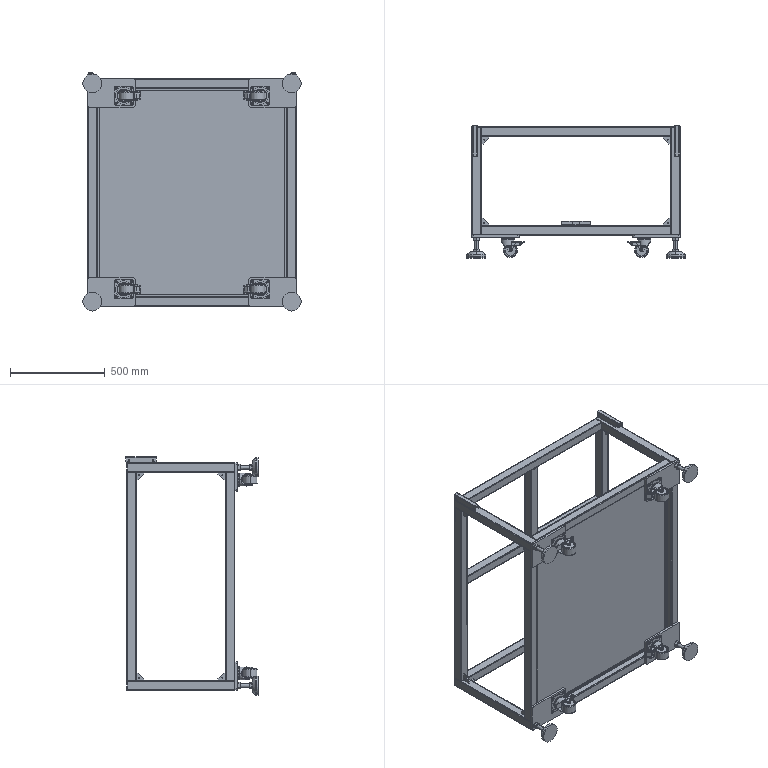Part | SolidWorks | features ReferencePattern 18, MirrorCompFeat 5 | 67 solids | 1566 faces | box 1150 x 697 x 1255 mm | volume 10713372 mm3 | plane 708 | cylinder 582 | cone 180 | spline 80 | torus 16 | commonest cylinder face diameters 4 x92 8 x92 5 x40 10 x40 20 x40 6.8 x32